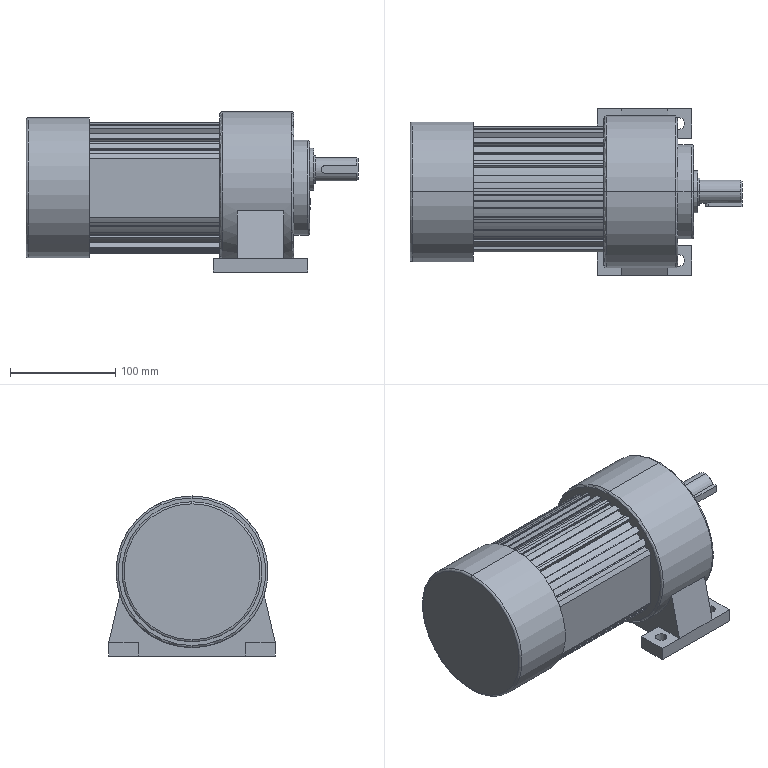Part | SolidWorks | features BaseBody 1 | 1 solid | 428 faces | box 315 x 158 x 152 mm | volume 3662443 mm3 | plane 187 | cylinder 167 | spline 63 | torus 8 | cone 3 | commonest cylinder face diameters 1 x43 8 x39 116 x24 124 x16 127 x16 11 x8